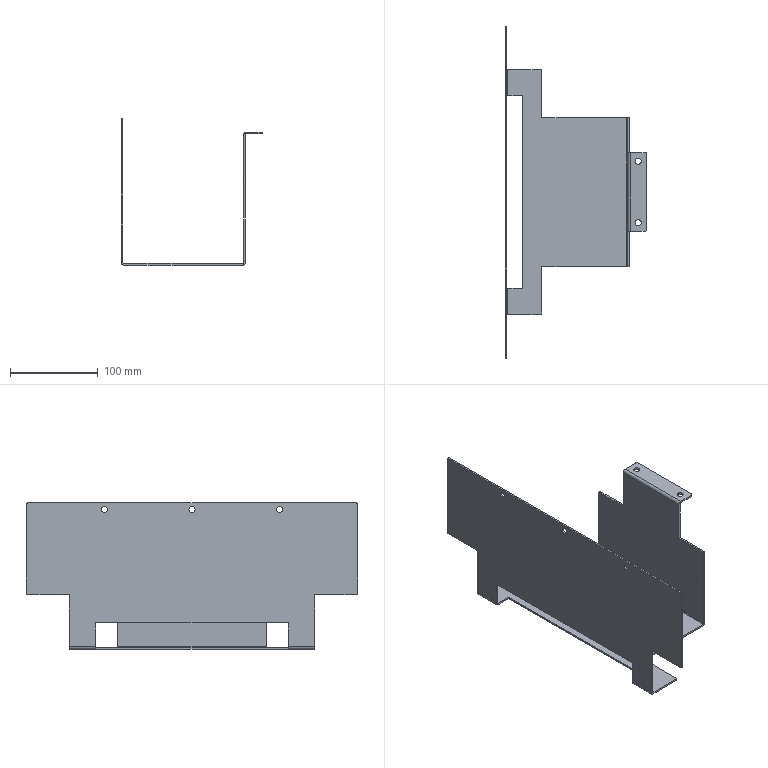Part | STEP file | PN_0009_default | 1 solid | 56 faces | box 162 x 379 x 167 mm | volume 195239 mm3 | cylinder 28 | plane 28 | commonest cylinder face diameters 4 x10 7 x10 2 x4 6 x4